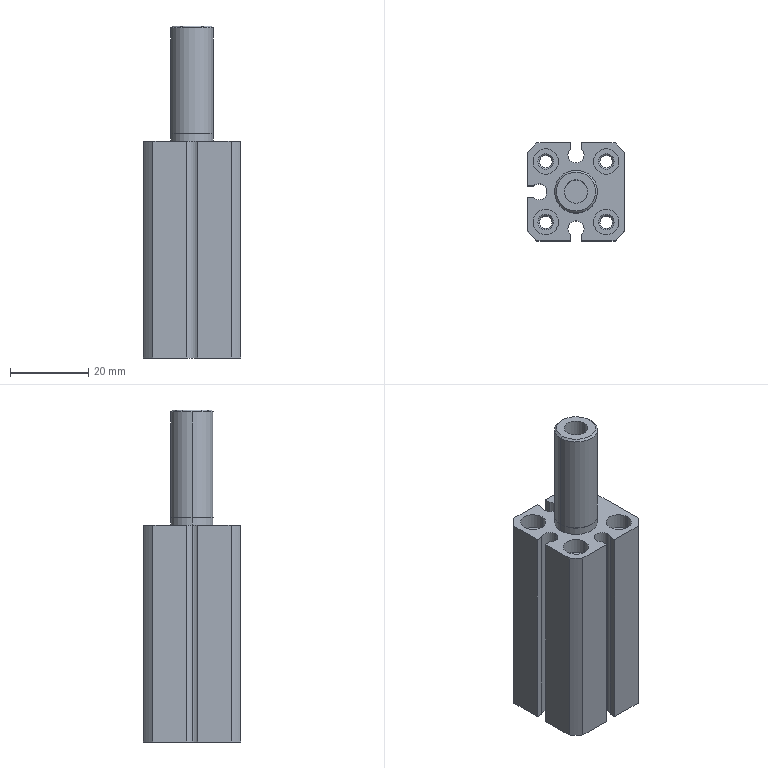Part | SolidWorks | features BaseBody 1 | 1 solid | 125 faces | box 25 x 25 x 85 mm | volume 25696 mm3 | cylinder 64 | plane 35 | cone 26 | commonest cylinder face diameters 3.242 x16 6.5 x16 3.5 x8 4.15 x8 4.134 x4 32 x4